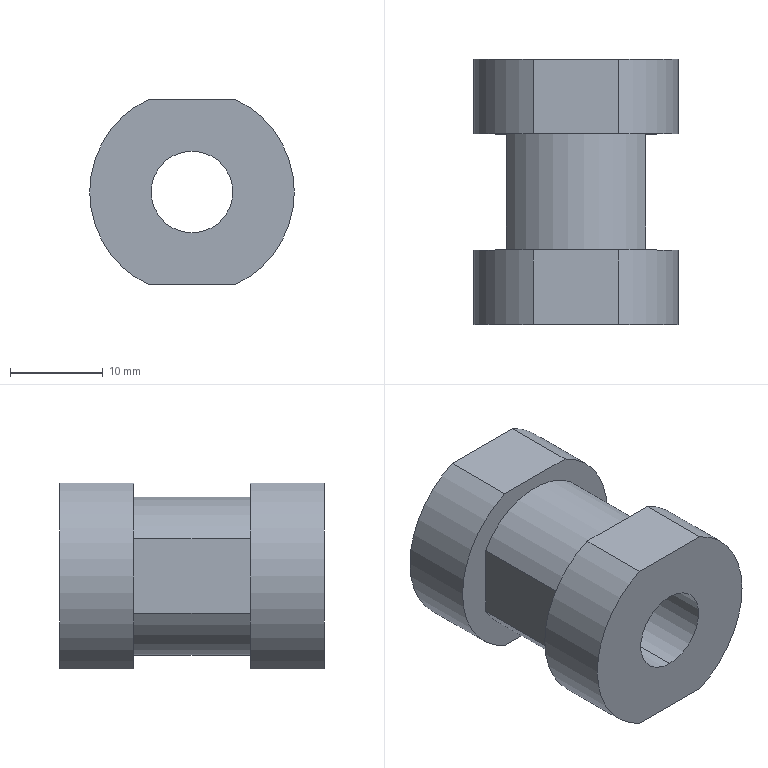Part | SolidWorks | features ICE 5, Extrusion 1, HoleWzd 1 | 1 solid | 19 faces | box 22 x 28.5 x 20 mm | volume 6854 mm3 | plane 10 | cylinder 9 | commonest cylinder face diameters 22 x4 17 x3 8.8 x2
STEP:
#1=CARTESIAN_POINT('',(0.,24.5,4.4));
#2=VERTEX_POINT('',#1);
#3=CARTESIAN_POINT('',(0.,24.5,-4.4));
#4=VERTEX_POINT('',#3);
#5=CARTESIAN_POINT('',(0.,24.5,0.));
#6=DIRECTION('',(0.,-1.,0.));
#7=DIRECTION('',(0.,0.,-1.));
#8=AXIS2_PLACEMENT_3D('',#5,#6,#7);
#9=CIRCLE('',#8,4.4);
#10=EDGE_CURVE('',#2,#4,#9,.T.);
#11=ORIENTED_EDGE('',*,*,#10,.F.);
#12=CARTESIAN_POINT('',(0.,-4.,4.4));
#13=VERTEX_POINT('',#12);
#14=CARTESIAN_POINT('',(0.,-4.,4.4));
#15=DIRECTION('',(0.,-1.,0.));
#16=VECTOR('',#15,1000.);
#17=LINE('',#14,#16);
#18=EDGE_CURVE('',#2,#13,#17,.T.);
#19=ORIENTED_EDGE('',*,*,#18,.T.);
#20=CARTESIAN_POINT('',(0.,-4.,-4.4));
#21=VERTEX_POINT('',#20);
#22=CARTESIAN_POINT('',(0.,-4.,0.));
#23=DIRECTION('',(0.,-1.,0.));
#24=DIRECTION('',(0.,0.,-1.));
#25=AXIS2_PLACEMENT_3D('',#22,#23,#24);
#26=CIRCLE('',#25,4.4);
#27=EDGE_CURVE('',#13,#21,#26,.T.);
#28=ORIENTED_EDGE('',*,*,#27,.T.);
#29=CARTESIAN_POINT('',(0.,-4.,-4.4));
#30=DIRECTION('',(0.,-1.,0.));
#31=VECTOR('',#30,1000.);
#32=LINE('',#29,#31);
#33=EDGE_CURVE('',#4,#21,#32,.T.);
#34=ORIENTED_EDGE('',*,*,#33,.F.);
#35=EDGE_LOOP('',(#11,#19,#28,#34));
#36=FACE_OUTER_BOUND('',#35,.T.);
#37=CARTESIAN_POINT('',(0.,-4.,0.));
#38=DIRECTION('',(0.,-1.,0.));
#39=DIRECTION('',(0.,0.,-1.));
#40=AXIS2_PLACEMENT_3D('',#37,#38,#39);
#41=CYLINDRICAL_SURFACE('',#40,4.4);
#42=ADVANCED_FACE('',(#36),#41,.F.);
#43=CARTESIAN_POINT('',(0.,16.5,-8.5));
#44=VERTEX_POINT('',#43);
#45=CARTESIAN_POINT('',(-7.5,16.5,-4.));
#46=VERTEX_POINT('',#45);
#47=CARTESIAN_POINT('',(0.,16.5,0.));
#48=DIRECTION('',(0.,1.,0.));
#49=DIRECTION('',(0.,0.,1.));
#50=AXIS2_PLACEMENT_3D('',#47,#48,#49);
#51=CIRCLE('',#50,8.5);
#52=EDGE_CURVE('',#44,#46,#51,.T.);
#53=ORIENTED_EDGE('',*,*,#52,.F.);
#54=CARTESIAN_POINT('',(0.,4.,-8.5));
#55=VERTEX_POINT('',#54);
#56=CARTESIAN_POINT('',(0.,16.5,-8.5));
#57=DIRECTION('',(0.,-1.,0.));
#58=VECTOR('',#57,1000.);
#59=LINE('',#56,#58);
#60=EDGE_CURVE('',#44,#55,#59,.T.);
#61=ORIENTED_EDGE('',*,*,#60,.T.);
#62=CARTESIAN_POINT('',(-7.5,4.,-4.));
#63=VERTEX_POINT('',#62);
#64=CARTESIAN_POINT('',(0.,4.,0.));
#65=DIRECTION('',(0.,1.,0.));
#66=DIRECTION('',(0.,0.,1.));
#67=AXIS2_PLACEMENT_3D('',#64,#65,#66);
#68=CIRCLE('',#67,8.5);
#69=EDGE_CURVE('',#55,#63,#68,.T.);
#70=ORIENTED_EDGE('',*,*,#69,.T.);
#71=CARTESIAN_POINT('',(-7.5,16.5,-4.));
#72=DIRECTION('',(0.,1.,0.));
#73=VECTOR('',#72,1000.);
#74=LINE('',#71,#73);
#75=EDGE_CURVE('',#63,#46,#74,.T.);
#76=ORIENTED_EDGE('',*,*,#75,.T.);
#77=EDGE_LOOP('',(#53,#61,#70,#76));
#78=FACE_OUTER_BOUND('',#77,.T.);
#79=CARTESIAN_POINT('',(0.,16.5,0.));
#80=DIRECTION('',(0.,-1.,0.));
#81=DIRECTION('',(0.,0.,-1.));
#82=AXIS2_PLACEMENT_3D('',#79,#80,#81);
#83=CYLINDRICAL_SURFACE('',#82,8.5);
#84=ADVANCED_FACE('',(#78),#83,.T.);
#85=CARTESIAN_POINT('',(-7.5,16.5,4.));
#86=VERTEX_POINT('',#85);
#87=CARTESIAN_POINT('',(7.5,16.5,4.));
#88=VERTEX_POINT('',#87);
#89=CARTESIAN_POINT('',(0.,16.5,0.));
#90=DIRECTION('',(0.,1.,0.));
#91=DIRECTION('',(0.,0.,1.));
#92=AXIS2_PLACEMENT_3D('',#89,#90,#91);
#93=CIRCLE('',#92,8.5);
#94=EDGE_CURVE('',#86,#88,#93,.T.);
#95=ORIENTED_EDGE('',*,*,#94,.F.);
#96=CARTESIAN_POINT('',(-7.5,4.,4.));
#97=VERTEX_POINT('',#96);
#98=CARTESIAN_POINT('',(-7.5,16.5,4.));
#99=DIRECTION('',(0.,-1.,0.));
#100=VECTOR('',#99,1000.);
#101=LINE('',#98,#100);
#102=EDGE_CURVE('',#86,#97,#101,.T.);
#103=ORIENTED_EDGE('',*,*,#102,.T.);
#104=CARTESIAN_POINT('',(7.5,4.,4.));
#105=VERTEX_POINT('',#104);
#106=CARTESIAN_POINT('',(0.,4.,0.));
#107=DIRECTION('',(0.,1.,0.));
#108=DIRECTION('',(0.,0.,1.));
#109=AXIS2_PLACEMENT_3D('',#106,#107,#108);
#110=CIRCLE('',#109,8.5);
#111=EDGE_CURVE('',#97,#105,#110,.T.);
#112=ORIENTED_EDGE('',*,*,#111,.T.);
#113=CARTESIAN_POINT('',(7.5,16.5,4.));
#114=DIRECTION('',(0.,1.,0.));
#115=VECTOR('',#114,1000.);
#116=LINE('',#113,#115);
#117=EDGE_CURVE('',#105,#88,#116,.T.);
#118=ORIENTED_EDGE('',*,*,#117,.T.);
#119=EDGE_LOOP('',(#95,#103,#112,#118));
#120=FACE_OUTER_BOUND('',#119,.T.);
#121=CARTESIAN_POINT('',(0.,16.5,0.));
#122=DIRECTION('',(0.,-1.,0.));
#123=DIRECTION('',(0.,0.,-1.));
#124=AXIS2_PLACEMENT_3D('',#121,#122,#123);
#125=CYLINDRICAL_SURFACE('',#124,8.5);
#126=ADVANCED_FACE('',(#120),#125,.T.);
#127=CARTESIAN_POINT('',(4.583,4.,10.));
#128=VERTEX_POINT('',#127);
#129=CARTESIAN_POINT('',(4.583,4.,-10.));
#130=VERTEX_POINT('',#129);
#131=CARTESIAN_POINT('',(0.,4.,0.));
#132=DIRECTION('',(0.,1.,0.));
#133=DIRECTION('',(0.,0.,1.));
#134=AXIS2_PLACEMENT_3D('',#131,#132,#133);
#135=CIRCLE('',#134,11.);
#136=EDGE_CURVE('',#128,#130,#135,.T.);
#137=ORIENTED_EDGE('',*,*,#136,.F.);
#138=CARTESIAN_POINT('',(4.583,-4.,10.));
#139=VERTEX_POINT('',#138);
#140=CARTESIAN_POINT('',(4.583,24.5,10.));
#141=DIRECTION('',(0.,-1.,0.));
#142=VECTOR('',#141,1000.);
#143=LINE('',#140,#142);
#144=EDGE_CURVE('',#128,#139,#143,.T.);
#145=ORIENTED_EDGE('',*,*,#144,.T.);
#146=CARTESIAN_POINT('',(4.583,-4.,-10.));
#147=VERTEX_POINT('',#146);
#148=CARTESIAN_POINT('',(0.,-4.,0.));
#149=DIRECTION('',(0.,1.,0.));
#150=DIRECTION('',(0.,0.,1.));
#151=AXIS2_PLACEMENT_3D('',#148,#149,#150);
#152=CIRCLE('',#151,11.);
#153=EDGE_CURVE('',#139,#147,#152,.T.);
#154=ORIENTED_EDGE('',*,*,#153,.T.);
#155=CARTESIAN_POINT('',(4.583,24.5,-10.));
#156=DIRECTION('',(0.,-1.,0.));
#157=VECTOR('',#156,1000.);
#158=LINE('',#155,#157);
#159=EDGE_CURVE('',#130,#147,#158,.T.);
#160=ORIENTED_EDGE('',*,*,#159,.F.);
#161=EDGE_LOOP('',(#137,#145,#154,#160));
#162=FACE_OUTER_BOUND('',#161,.T.);
#163=CARTESIAN_POINT('',(0.,4.,0.));
#164=DIRECTION('',(0.,-1.,0.));
#165=DIRECTION('',(0.,0.,-1.));
#166=AXIS2_PLACEMENT_3D('',#163,#164,#165);
#167=CYLINDRICAL_SURFACE('',#166,11.);
#168=ADVANCED_FACE('',(#162),#167,.T.);
#169=CARTESIAN_POINT('',(4.583,24.5,10.));
#170=VERTEX_POINT('',#169);
#171=CARTESIAN_POINT('',(4.583,24.5,-10.));
#172=VERTEX_POINT('',#171);
#173=CARTESIAN_POINT('',(0.,24.5,0.));
#174=DIRECTION('',(0.,1.,0.));
#175=DIRECTION('',(0.,0.,1.));
#176=AXIS2_PLACEMENT_3D('',#173,#174,#175);
#177=CIRCLE('',#176,11.);
#178=EDGE_CURVE('',#170,#172,#177,.T.);
#179=ORIENTED_EDGE('',*,*,#178,.F.);
#180=CARTESIAN_POINT('',(4.583,16.5,10.));
#181=VERTEX_POINT('',#180);
#182=CARTESIAN_POINT('',(4.583,24.5,10.));
#183=DIRECTION('',(0.,-1.,0.));
#184=VECTOR('',#183,1000.);
#185=LINE('',#182,#184);
#186=EDGE_CURVE('',#170,#181,#185,.T.);
#187=ORIENTED_EDGE('',*,*,#186,.T.);
#188=CARTESIAN_POINT('',(4.583,16.5,-10.));
#189=VERTEX_POINT('',#188);
#190=CARTESIAN_POINT('',(0.,16.5,0.));
#191=DIRECTION('',(0.,1.,0.));
#192=DIRECTION('',(0.,0.,1.));
#193=AXIS2_PLACEMENT_3D('',#190,#191,#192);
#194=CIRCLE('',#193,11.);
#195=EDGE_CURVE('',#181,#189,#194,.T.);
#196=ORIENTED_EDGE('',*,*,#195,.T.);
#197=CARTESIAN_POINT('',(4.583,24.5,-10.));
#198=DIRECTION('',(0.,-1.,0.));
#199=VECTOR('',#198,1000.);
#200=LINE('',#197,#199);
#201=EDGE_CURVE('',#172,#189,#200,.T.);
#202=ORIENTED_EDGE('',*,*,#201,.F.);
#203=EDGE_LOOP('',(#179,#187,#196,#202));
#204=FACE_OUTER_BOUND('',#203,.T.);
#205=CARTESIAN_POINT('',(0.,24.5,0.));
#206=DIRECTION('',(0.,-1.,0.));
#207=DIRECTION('',(0.,0.,-1.));
#208=AXIS2_PLACEMENT_3D('',#205,#206,#207);
#209=CYLINDRICAL_SURFACE('',#208,11.);
#210=ADVANCED_FACE('',(#204),#209,.T.);
#211=CARTESIAN_POINT('',(-4.583,-4.,-10.));
#212=VERTEX_POINT('',#211);
#213=CARTESIAN_POINT('',(-4.583,-4.,10.));
#214=VERTEX_POINT('',#213);
#215=CARTESIAN_POINT('',(0.,-4.,0.));
#216=DIRECTION('',(0.,1.,0.));
#217=DIRECTION('',(0.,0.,1.));
#218=AXIS2_PLACEMENT_3D('',#215,#216,#217);
#219=CIRCLE('',#218,11.);
#220=EDGE_CURVE('',#212,#214,#219,.T.);
#221=ORIENTED_EDGE('',*,*,#220,.T.);
#222=CARTESIAN_POINT('',(-4.583,4.,10.));
#223=VERTEX_POINT('',#222);
#224=CARTESIAN_POINT('',(-4.583,24.5,10.));
#225=DIRECTION('',(0.,-1.,0.));
#226=VECTOR('',#225,1000.);
#227=LINE('',#224,#226);
#228=EDGE_CURVE('',#223,#214,#227,.T.);
#229=ORIENTED_EDGE('',*,*,#228,.F.);
#230=CARTESIAN_POINT('',(-4.583,4.,-10.));
#231=VERTEX_POINT('',#230);
#232=CARTESIAN_POINT('',(0.,4.,0.));
#233=DIRECTION('',(0.,1.,0.));
#234=DIRECTION('',(0.,0.,1.));
#235=AXIS2_PLACEMENT_3D('',#232,#233,#234);
#236=CIRCLE('',#235,11.);
#237=EDGE_CURVE('',#231,#223,#236,.T.);
#238=ORIENTED_EDGE('',*,*,#237,.F.);
#239=CARTESIAN_POINT('',(-4.583,24.5,-10.));
#240=DIRECTION('',(0.,-1.,0.));
#241=VECTOR('',#240,1000.);
#242=LINE('',#239,#241);
#243=EDGE_CURVE('',#231,#212,#242,.T.);
#244=ORIENTED_EDGE('',*,*,#243,.T.);
#245=EDGE_LOOP('',(#221,#229,#238,#244));
#246=FACE_OUTER_BOUND('',#245,.T.);
#247=CARTESIAN_POINT('',(0.,4.,0.));
#248=DIRECTION('',(0.,-1.,0.));
#249=DIRECTION('',(0.,0.,-1.));
#250=AXIS2_PLACEMENT_3D('',#247,#248,#249);
#251=CYLINDRICAL_SURFACE('',#250,11.);
#252=ADVANCED_FACE('',(#246),#251,.T.);
#253=ORIENTED_EDGE('',*,*,#111,.F.);
#254=CARTESIAN_POINT('',(-7.5,4.,-24.5));
#255=DIRECTION('',(0.,0.,1.));
#256=VECTOR('',#255,1000.);
#257=LINE('',#254,#256);
#258=EDGE_CURVE('',#63,#97,#257,.T.);
#259=ORIENTED_EDGE('',*,*,#258,.F.);
#260=ORIENTED_EDGE('',*,*,#69,.F.);
#261=CARTESIAN_POINT('',(7.5,4.,-4.));
#262=VERTEX_POINT('',#261);
#263=CARTESIAN_POINT('',(0.,4.,0.));
#264=DIRECTION('',(0.,1.,0.));
#265=DIRECTION('',(0.,0.,1.));
#266=AXIS2_PLACEMENT_3D('',#263,#264,#265);
#267=CIRCLE('',#266,8.5);
#268=EDGE_CURVE('',#262,#55,#267,.T.);
#269=ORIENTED_EDGE('',*,*,#268,.F.);
#270=CARTESIAN_POINT('',(7.5,4.,-24.5));
#271=DIRECTION('',(0.,0.,1.));
#272=VECTOR('',#271,1000.);
#273=LINE('',#270,#272);
#274=EDGE_CURVE('',#262,#105,#273,.T.);
#275=ORIENTED_EDGE('',*,*,#274,.T.);
#276=EDGE_LOOP('',(#253,#259,#260,#269,#275));
#277=FACE_BOUND('',#276,.T.);
#278=ORIENTED_EDGE('',*,*,#136,.T.);
#279=CARTESIAN_POINT('',(0.,4.,-10.));
#280=DIRECTION('',(1.,0.,0.));
#281=VECTOR('',#280,1000.);
#282=LINE('',#279,#281);
#283=EDGE_CURVE('',#231,#130,#282,.T.);
#284=ORIENTED_EDGE('',*,*,#283,.F.);
#285=ORIENTED_EDGE('',*,*,#237,.T.);
#286=CARTESIAN_POINT('',(0.,4.,10.));
#287=DIRECTION('',(-1.,0.,0.));
#288=VECTOR('',#287,1000.);
#289=LINE('',#286,#288);
#290=EDGE_CURVE('',#128,#223,#289,.T.);
#291=ORIENTED_EDGE('',*,*,#290,.F.);
#292=EDGE_LOOP('',(#278,#284,#285,#291));
#293=FACE_OUTER_BOUND('',#292,.T.);
#294=CARTESIAN_POINT('',(0.,4.,0.));
#295=DIRECTION('',(0.,1.,0.));
#296=DIRECTION('',(0.,0.,1.));
#297=AXIS2_PLACEMENT_3D('',#294,#295,#296);
#298=PLANE('',#297);
#299=ADVANCED_FACE('',(#277,#293),#298,.T.);
#300=CARTESIAN_POINT('',(0.,-4.,0.));
#301=DIRECTION('',(0.,-1.,0.));
#302=DIRECTION('',(0.,0.,-1.));
#303=AXIS2_PLACEMENT_3D('',#300,#301,#302);
#304=CIRCLE('',#303,4.4);
#305=EDGE_CURVE('',#21,#13,#304,.T.);
#306=ORIENTED_EDGE('',*,*,#305,.F.);
#307=ORIENTED_EDGE('',*,*,#27,.F.);
#308=EDGE_LOOP('',(#306,#307));
#309=FACE_BOUND('',#308,.T.);
#310=ORIENTED_EDGE('',*,*,#153,.F.);
#311=CARTESIAN_POINT('',(-4.583,-4.,10.));
#312=DIRECTION('',(1.,0.,0.));
#313=VECTOR('',#312,1000.);
#314=LINE('',#311,#313);
#315=EDGE_CURVE('',#214,#139,#314,.T.);
#316=ORIENTED_EDGE('',*,*,#315,.F.);
#317=ORIENTED_EDGE('',*,*,#220,.F.);
#318=CARTESIAN_POINT('',(-4.583,-4.,-10.));
#319=DIRECTION('',(-1.,0.,0.));
#320=VECTOR('',#319,1000.);
#321=LINE('',#318,#320);
#322=EDGE_CURVE('',#147,#212,#321,.T.);
#323=ORIENTED_EDGE('',*,*,#322,.F.);
#324=EDGE_LOOP('',(#310,#316,#317,#323));
#325=FACE_OUTER_BOUND('',#324,.T.);
#326=CARTESIAN_POINT('',(0.,-4.,0.));
#327=DIRECTION('',(0.,1.,0.));
#328=DIRECTION('',(0.,0.,1.));
#329=AXIS2_PLACEMENT_3D('',#326,#327,#328);
#330=PLANE('',#329);
#331=ADVANCED_FACE('',(#309,#325),#330,.F.);
#332=ORIENTED_EDGE('',*,*,#60,.F.);
#333=CARTESIAN_POINT('',(7.5,16.5,-4.));
#334=VERTEX_POINT('',#333);
#335=CARTESIAN_POINT('',(0.,16.5,0.));
#336=DIRECTION('',(0.,1.,0.));
#337=DIRECTION('',(0.,0.,1.));
#338=AXIS2_PLACEMENT_3D('',#335,#336,#337);
#339=CIRCLE('',#338,8.5);
#340=EDGE_CURVE('',#334,#44,#339,.T.);
#341=ORIENTED_EDGE('',*,*,#340,.F.);
#342=CARTESIAN_POINT('',(7.5,16.5,-4.));
#343=DIRECTION('',(0.,-1.,0.));
#344=VECTOR('',#343,1000.);
#345=LINE('',#342,#344);
#346=EDGE_CURVE('',#334,#262,#345,.T.);
#347=ORIENTED_EDGE('',*,*,#346,.T.);
#348=ORIENTED_EDGE('',*,*,#268,.T.);
#349=EDGE_LOOP('',(#332,#341,#347,#348));
#350=FACE_OUTER_BOUND('',#349,.T.);
#351=CARTESIAN_POINT('',(0.,16.5,0.));
#352=DIRECTION('',(0.,-1.,0.));
#353=DIRECTION('',(0.,0.,-1.));
#354=AXIS2_PLACEMENT_3D('',#351,#352,#353);
#355=CYLINDRICAL_SURFACE('',#354,8.5);
#356=ADVANCED_FACE('',(#350),#355,.T.);
#357=CARTESIAN_POINT('',(-4.583,16.5,-10.));
#358=VERTEX_POINT('',#357);
#359=CARTESIAN_POINT('',(-4.583,16.5,10.));
#360=VERTEX_POINT('',#359);
#361=CARTESIAN_POINT('',(0.,16.5,0.));
#362=DIRECTION('',(0.,1.,0.));
#363=DIRECTION('',(0.,0.,1.));
#364=AXIS2_PLACEMENT_3D('',#361,#362,#363);
#365=CIRCLE('',#364,11.);
#366=EDGE_CURVE('',#358,#360,#365,.T.);
#367=ORIENTED_EDGE('',*,*,#366,.T.);
#368=CARTESIAN_POINT('',(-4.583,24.5,10.));
#369=VERTEX_POINT('',#368);
#370=CARTESIAN_POINT('',(-4.583,24.5,10.));
#371=DIRECTION('',(0.,-1.,0.));
#372=VECTOR('',#371,1000.);
#373=LINE('',#370,#372);
#374=EDGE_CURVE('',#369,#360,#373,.T.);
#375=ORIENTED_EDGE('',*,*,#374,.F.);
#376=CARTESIAN_POINT('',(-4.583,24.5,-10.));
#377=VERTEX_POINT('',#376);
#378=CARTESIAN_POINT('',(0.,24.5,0.));
#379=DIRECTION('',(0.,1.,0.));
#380=DIRECTION('',(0.,0.,1.));
#381=AXIS2_PLACEMENT_3D('',#378,#379,#380);
#382=CIRCLE('',#381,11.);
#383=EDGE_CURVE('',#377,#369,#382,.T.);
#384=ORIENTED_EDGE('',*,*,#383,.F.);
#385=CARTESIAN_POINT('',(-4.583,24.5,-10.));
#386=DIRECTION('',(0.,-1.,0.));
#387=VECTOR('',#386,1000.);
#388=LINE('',#385,#387);
#389=EDGE_CURVE('',#377,#358,#388,.T.);
#390=ORIENTED_EDGE('',*,*,#389,.T.);
#391=EDGE_LOOP('',(#367,#375,#384,#390));
#392=FACE_OUTER_BOUND('',#391,.T.);
#393=CARTESIAN_POINT('',(0.,24.5,0.));
#394=DIRECTION('',(0.,-1.,0.));
#395=DIRECTION('',(0.,0.,-1.));
#396=AXIS2_PLACEMENT_3D('',#393,#394,#395);
#397=CYLINDRICAL_SURFACE('',#396,11.);
#398=ADVANCED_FACE('',(#392),#397,.T.);
#399=CARTESIAN_POINT('',(-4.583,24.5,10.));
#400=DIRECTION('',(1.,0.,0.));
#401=VECTOR('',#400,1000.);
#402=LINE('',#399,#401);
#403=EDGE_CURVE('',#369,#170,#402,.T.);
#404=ORIENTED_EDGE('',*,*,#403,.T.);
#405=ORIENTED_EDGE('',*,*,#178,.T.);
#406=CARTESIAN_POINT('',(-4.583,24.5,-10.));
#407=DIRECTION('',(-1.,0.,0.));
#408=VECTOR('',#407,1000.);
#409=LINE('',#406,#408);
#410=EDGE_CURVE('',#172,#377,#409,.T.);
#411=ORIENTED_EDGE('',*,*,#410,.T.);
#412=ORIENTED_EDGE('',*,*,#383,.T.);
#413=EDGE_LOOP('',(#404,#405,#411,#412));
#414=FACE_OUTER_BOUND('',#413,.T.);
#415=CARTESIAN_POINT('',(0.,24.5,0.));
#416=DIRECTION('',(0.,-1.,0.));
#417=DIRECTION('',(0.,0.,-1.));
#418=AXIS2_PLACEMENT_3D('',#415,#416,#417);
#419=CIRCLE('',#418,4.4);
#420=EDGE_CURVE('',#4,#2,#419,.T.);
#421=ORIENTED_EDGE('',*,*,#420,.T.);
#422=ORIENTED_EDGE('',*,*,#10,.T.);
#423=EDGE_LOOP('',(#421,#422));
#424=FACE_BOUND('',#423,.T.);
#425=CARTESIAN_POINT('',(0.,24.5,0.));
#426=DIRECTION('',(0.,1.,0.));
#427=DIRECTION('',(0.,0.,1.));
#428=AXIS2_PLACEMENT_3D('',#425,#426,#427);
#429=PLANE('',#428);
#430=ADVANCED_FACE('',(#414,#424),#429,.T.);
#431=ORIENTED_EDGE('',*,*,#340,.T.);
#432=ORIENTED_EDGE('',*,*,#52,.T.);
#433=CARTESIAN_POINT('',(-7.5,16.5,-24.5));
#434=DIRECTION('',(0.,0.,1.));
#435=VECTOR('',#434,1000.);
#436=LINE('',#433,#435);
#437=EDGE_CURVE('',#46,#86,#436,.T.);
#438=ORIENTED_EDGE('',*,*,#437,.T.);
#439=ORIENTED_EDGE('',*,*,#94,.T.);
#440=CARTESIAN_POINT('',(7.5,16.5,-24.5));
#441=DIRECTION('',(0.,0.,1.));
#442=VECTOR('',#441,1000.);
#443=LINE('',#440,#442);
#444=EDGE_CURVE('',#334,#88,#443,.T.);
#445=ORIENTED_EDGE('',*,*,#444,.F.);
#446=EDGE_LOOP('',(#431,#432,#438,#439,#445));
#447=FACE_BOUND('',#446,.T.);
#448=CARTESIAN_POINT('',(0.,16.5,-10.));
#449=DIRECTION('',(1.,0.,0.));
#450=VECTOR('',#449,1000.);
#451=LINE('',#448,#450);
#452=EDGE_CURVE('',#358,#189,#451,.T.);
#453=ORIENTED_EDGE('',*,*,#452,.T.);
#454=ORIENTED_EDGE('',*,*,#195,.F.);
#455=CARTESIAN_POINT('',(0.,16.5,10.));
#456=DIRECTION('',(-1.,0.,0.));
#457=VECTOR('',#456,1000.);
#458=LINE('',#455,#457);
#459=EDGE_CURVE('',#181,#360,#458,.T.);
#460=ORIENTED_EDGE('',*,*,#459,.T.);
#461=ORIENTED_EDGE('',*,*,#366,.F.);
#462=EDGE_LOOP('',(#453,#454,#460,#461));
#463=FACE_OUTER_BOUND('',#462,.T.);
#464=CARTESIAN_POINT('',(0.,16.5,0.));
#465=DIRECTION('',(0.,1.,0.));
#466=DIRECTION('',(0.,0.,1.));
#467=AXIS2_PLACEMENT_3D('',#464,#465,#466);
#468=PLANE('',#467);
#469=ADVANCED_FACE('',(#447,#463),#468,.F.);
#470=ORIENTED_EDGE('',*,*,#18,.F.);
#471=ORIENTED_EDGE('',*,*,#420,.F.);
#472=ORIENTED_EDGE('',*,*,#33,.T.);
#473=ORIENTED_EDGE('',*,*,#305,.T.);
#474=EDGE_LOOP('',(#470,#471,#472,#473));
#475=FACE_OUTER_BOUND('',#474,.T.);
#476=CARTESIAN_POINT('',(0.,-4.,0.));
#477=DIRECTION('',(0.,-1.,0.));
#478=DIRECTION('',(0.,0.,-1.));
#479=AXIS2_PLACEMENT_3D('',#476,#477,#478);
#480=CYLINDRICAL_SURFACE('',#479,4.4);
#481=ADVANCED_FACE('',(#475),#480,.F.);
#482=ORIENTED_EDGE('',*,*,#389,.F.);
#483=ORIENTED_EDGE('',*,*,#410,.F.);
#484=ORIENTED_EDGE('',*,*,#201,.T.);
#485=ORIENTED_EDGE('',*,*,#452,.F.);
#486=EDGE_LOOP('',(#482,#483,#484,#485));
#487=FACE_OUTER_BOUND('',#486,.T.);
#488=CARTESIAN_POINT('',(-4.583,24.5,-10.));
#489=DIRECTION('',(0.,0.,1.));
#490=DIRECTION('',(1.,0.,0.));
#491=AXIS2_PLACEMENT_3D('',#488,#489,#490);
#492=PLANE('',#491);
#493=ADVANCED_FACE('',(#487),#492,.F.);
#494=ORIENTED_EDGE('',*,*,#186,.F.);
#495=ORIENTED_EDGE('',*,*,#403,.F.);
#496=ORIENTED_EDGE('',*,*,#374,.T.);
#497=ORIENTED_EDGE('',*,*,#459,.F.);
#498=EDGE_LOOP('',(#494,#495,#496,#497));
#499=FACE_OUTER_BOUND('',#498,.T.);
#500=CARTESIAN_POINT('',(-4.583,24.5,10.));
#501=DIRECTION('',(0.,0.,-1.));
#502=DIRECTION('',(-1.,0.,0.));
#503=AXIS2_PLACEMENT_3D('',#500,#501,#502);
#504=PLANE('',#503);
#505=ADVANCED_FACE('',(#499),#504,.F.);
#506=ORIENTED_EDGE('',*,*,#283,.T.);
#507=ORIENTED_EDGE('',*,*,#159,.T.);
#508=ORIENTED_EDGE('',*,*,#322,.T.);
#509=ORIENTED_EDGE('',*,*,#243,.F.);
#510=EDGE_LOOP('',(#506,#507,#508,#509));
#511=FACE_OUTER_BOUND('',#510,.T.);
#512=CARTESIAN_POINT('',(-4.583,24.5,-10.));
#513=DIRECTION('',(0.,0.,1.));
#514=DIRECTION('',(1.,0.,0.));
#515=AXIS2_PLACEMENT_3D('',#512,#513,#514);
#516=PLANE('',#515);
#517=ADVANCED_FACE('',(#511),#516,.F.);
#518=ORIENTED_EDGE('',*,*,#290,.T.);
#519=ORIENTED_EDGE('',*,*,#228,.T.);
#520=ORIENTED_EDGE('',*,*,#315,.T.);
#521=ORIENTED_EDGE('',*,*,#144,.F.);
#522=EDGE_LOOP('',(#518,#519,#520,#521));
#523=FACE_OUTER_BOUND('',#522,.T.);
#524=CARTESIAN_POINT('',(-4.583,24.5,10.));
#525=DIRECTION('',(0.,0.,-1.));
#526=DIRECTION('',(-1.,0.,0.));
#527=AXIS2_PLACEMENT_3D('',#524,#525,#526);
#528=PLANE('',#527);
#529=ADVANCED_FACE('',(#523),#528,.F.);
#530=ORIENTED_EDGE('',*,*,#444,.T.);
#531=ORIENTED_EDGE('',*,*,#117,.F.);
#532=ORIENTED_EDGE('',*,*,#274,.F.);
#533=ORIENTED_EDGE('',*,*,#346,.F.);
#534=EDGE_LOOP('',(#530,#531,#532,#533));
#535=FACE_OUTER_BOUND('',#534,.T.);
#536=CARTESIAN_POINT('',(7.5,4.,-24.5));
#537=DIRECTION('',(-1.,0.,0.));
#538=DIRECTION('',(0.,-1.,0.));
#539=AXIS2_PLACEMENT_3D('',#536,#537,#538);
#540=PLANE('',#539);
#541=ADVANCED_FACE('',(#535),#540,.F.);
#542=ORIENTED_EDGE('',*,*,#437,.F.);
#543=ORIENTED_EDGE('',*,*,#75,.F.);
#544=ORIENTED_EDGE('',*,*,#258,.T.);
#545=ORIENTED_EDGE('',*,*,#102,.F.);
#546=EDGE_LOOP('',(#542,#543,#544,#545));
#547=FACE_OUTER_BOUND('',#546,.T.);
#548=CARTESIAN_POINT('',(-7.5,4.,-24.5));
#549=DIRECTION('',(1.,0.,0.));
#550=DIRECTION('',(0.,0.,-1.));
#551=AXIS2_PLACEMENT_3D('',#548,#549,#550);
#552=PLANE('',#551);
#553=ADVANCED_FACE('',(#547),#552,.F.);
#554=CLOSED_SHELL('',(#42,#84,#126,#168,#210,#252,#299,#331,#356,#398,#430,#469,#481,#493,#505,#517,#529,#541,#553));
#555=MANIFOLD_SOLID_BREP('',#554);
#556=CARTESIAN_POINT('',(0.,0.,0.));
#557=DIRECTION('',(0.,0.,1.));
#558=DIRECTION('',(1.,0.,0.));
#559=AXIS2_PLACEMENT_3D('',#556,#557,#558);
#560=(LENGTH_UNIT()NAMED_UNIT(*)SI_UNIT(.MILLI.,.METRE.));
#561=UNCERTAINTY_MEASURE_WITH_UNIT(LENGTH_MEASURE(0.00001),#560,'','');
#562=(NAMED_UNIT(*)PLANE_ANGLE_UNIT()SI_UNIT($,.RADIAN.));
#563=(NAMED_UNIT(*)SI_UNIT($,.STERADIAN.)SOLID_ANGLE_UNIT());
#564=(GEOMETRIC_REPRESENTATION_CONTEXT(3)GLOBAL_UNCERTAINTY_ASSIGNED_CONTEXT((#561))GLOBAL_UNIT_ASSIGNED_CONTEXT((#560,#562,#563))REPRESENTATION_CONTEXT('',''));
#565=ADVANCED_BREP_SHAPE_REPRESENTATION('',(#555,#559),#564);